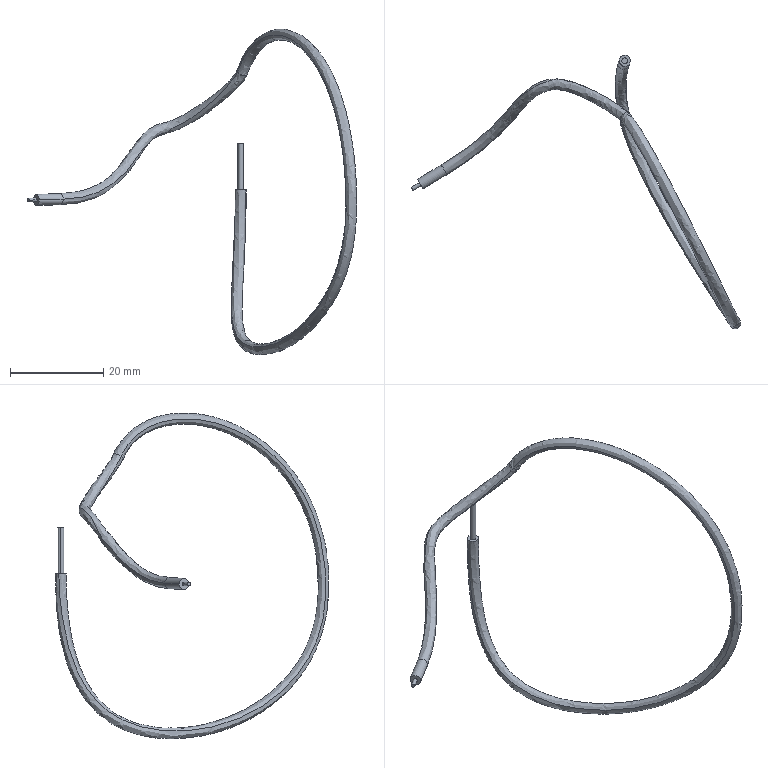Part | SolidWorks | features 3DProfileFeature 2, ICE 2, Sweep 1 | 1 solid | 14 faces | box 70.611 x 58.67 x 69.854 mm | volume 1093 mm3 | cylinder 6 | spline 4 | plane 4 | commonest cylinder face diameters 0.8 x2 1.237 x2 2.4 x2